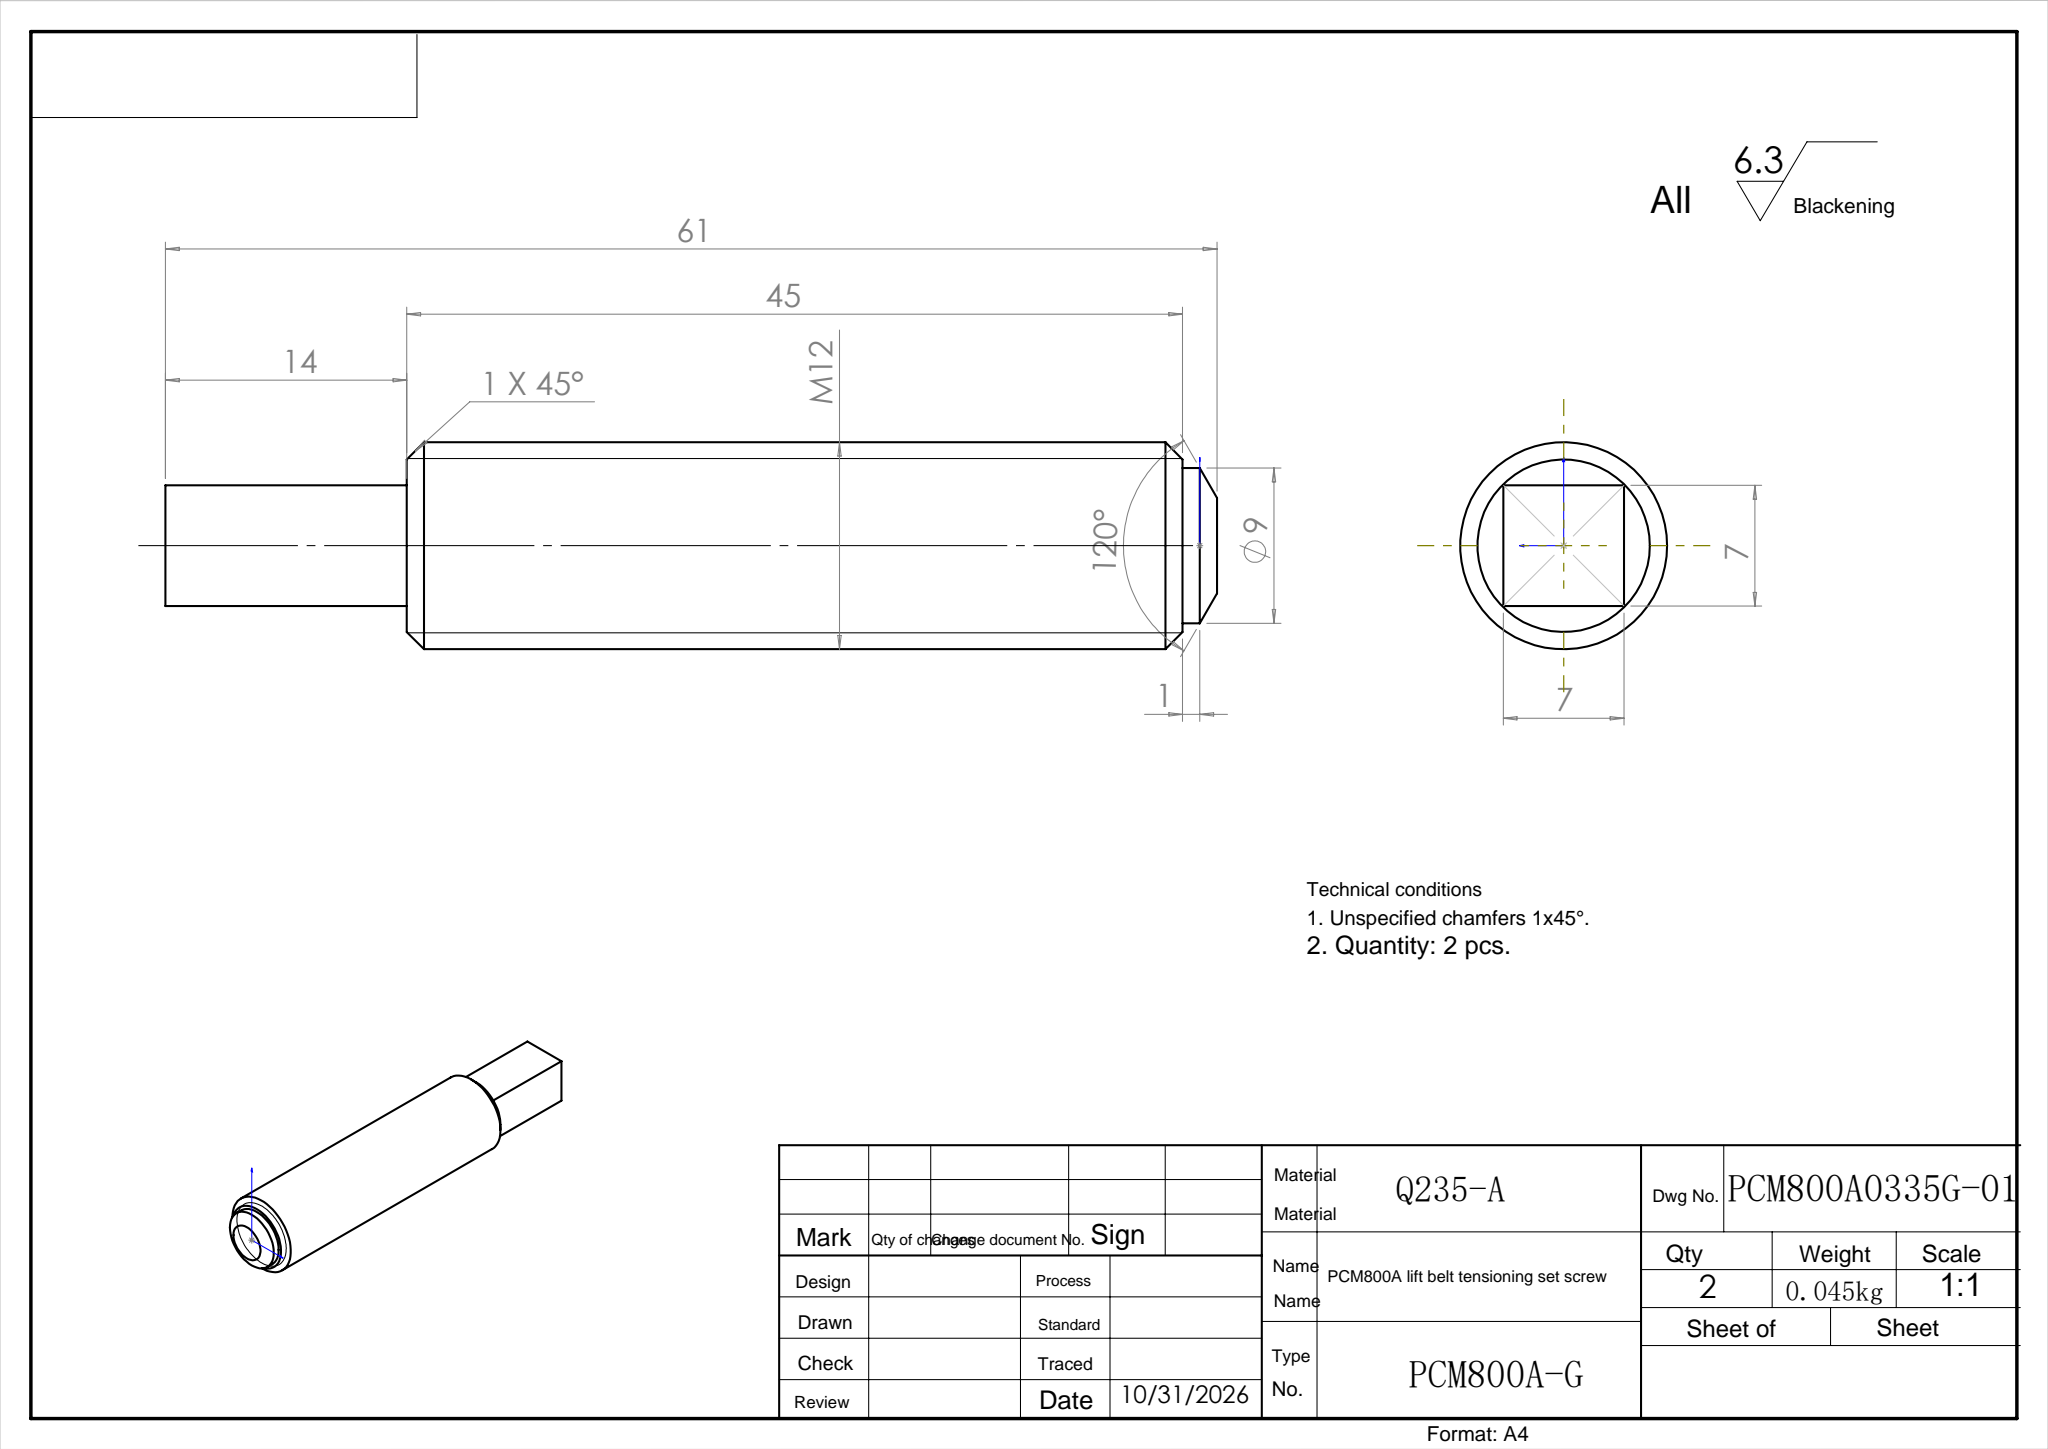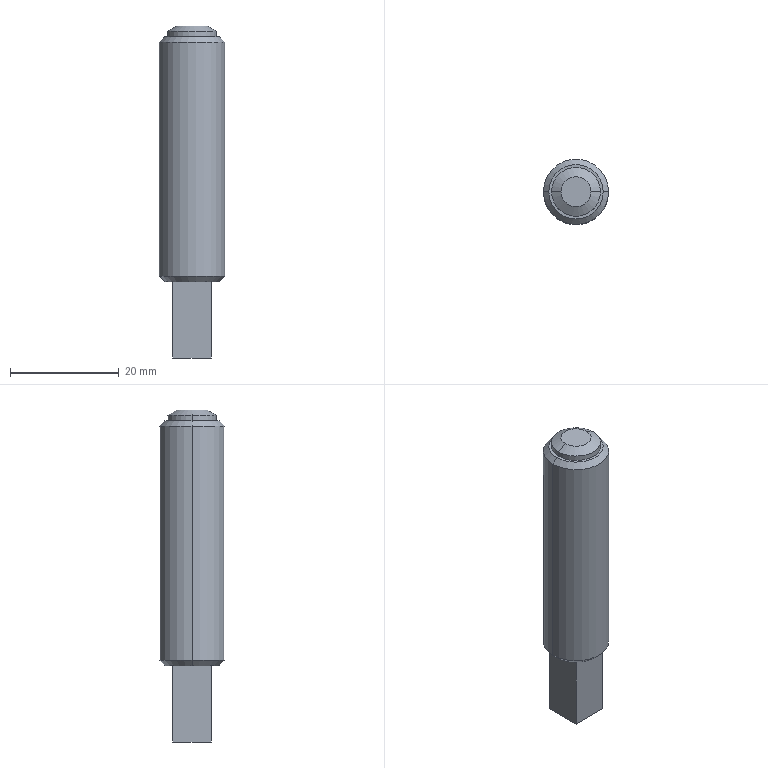Part | SolidWorks | features ICE 3, Chamfer 2, MirrorStock 1 | 1 solid | 18 faces | box 12 x 12 x 61 mm | volume 5846 mm3 | plane 8 | cone 6 | cylinder 4 | commonest cylinder face diameters 9 x2 12 x2
STEP:
#1=CARTESIAN_POINT('',(5.,0.,-1.));
#2=VERTEX_POINT('',#1);
#3=CARTESIAN_POINT('',(-5.,0.,-1.));
#4=VERTEX_POINT('',#3);
#5=CARTESIAN_POINT('',(0.,0.,-1.));
#6=DIRECTION('',(0.,0.,1.));
#7=DIRECTION('',(-1.,0.,0.));
#8=AXIS2_PLACEMENT_3D('',#5,#6,#7);
#9=CIRCLE('',#8,5.);
#10=EDGE_CURVE('',#2,#4,#9,.T.);
#11=ORIENTED_EDGE('',*,*,#10,.F.);
#12=CARTESIAN_POINT('',(6.,0.,-2.));
#13=VERTEX_POINT('',#12);
#14=CARTESIAN_POINT('',(5.,0.,-1.));
#15=DIRECTION('',(0.7071,0.,-0.7071));
#16=VECTOR('',#15,1000.);
#17=LINE('',#14,#16);
#18=EDGE_CURVE('',#2,#13,#17,.T.);
#19=ORIENTED_EDGE('',*,*,#18,.T.);
#20=CARTESIAN_POINT('',(-6.,0.,-2.));
#21=VERTEX_POINT('',#20);
#22=CARTESIAN_POINT('',(0.,0.,-2.));
#23=DIRECTION('',(0.,0.,-1.));
#24=DIRECTION('',(-1.,0.,0.));
#25=AXIS2_PLACEMENT_3D('',#22,#23,#24);
#26=CIRCLE('',#25,6.);
#27=EDGE_CURVE('',#21,#13,#26,.T.);
#28=ORIENTED_EDGE('',*,*,#27,.F.);
#29=CARTESIAN_POINT('',(-5.,0.,-1.));
#30=DIRECTION('',(-0.7071,0.,-0.7071));
#31=VECTOR('',#30,1000.);
#32=LINE('',#29,#31);
#33=EDGE_CURVE('',#4,#21,#32,.T.);
#34=ORIENTED_EDGE('',*,*,#33,.F.);
#35=EDGE_LOOP('',(#11,#19,#28,#34));
#36=FACE_OUTER_BOUND('',#35,.T.);
#37=CARTESIAN_POINT('',(0.,0.,-1.));
#38=DIRECTION('',(0.,0.,-1.));
#39=DIRECTION('',(-1.,0.,0.));
#40=AXIS2_PLACEMENT_3D('',#37,#38,#39);
#41=CONICAL_SURFACE('',#40,5.,0.7854);
#42=ADVANCED_FACE('',(#36),#41,.T.);
#43=CARTESIAN_POINT('',(-4.5,0.,-1.));
#44=VERTEX_POINT('',#43);
#45=CARTESIAN_POINT('',(4.5,0.,-1.));
#46=VERTEX_POINT('',#45);
#47=CARTESIAN_POINT('',(0.,0.,-1.));
#48=DIRECTION('',(0.,0.,1.));
#49=DIRECTION('',(1.,0.,0.));
#50=AXIS2_PLACEMENT_3D('',#47,#48,#49);
#51=CIRCLE('',#50,4.5);
#52=EDGE_CURVE('',#44,#46,#51,.T.);
#53=ORIENTED_EDGE('',*,*,#52,.T.);
#54=CARTESIAN_POINT('',(4.5,0.,0.));
#55=VERTEX_POINT('',#54);
#56=CARTESIAN_POINT('',(4.5,0.,-1.));
#57=DIRECTION('',(0.,0.,1.));
#58=VECTOR('',#57,1000.);
#59=LINE('',#56,#58);
#60=EDGE_CURVE('',#46,#55,#59,.T.);
#61=ORIENTED_EDGE('',*,*,#60,.T.);
#62=CARTESIAN_POINT('',(-4.5,0.,0.));
#63=VERTEX_POINT('',#62);
#64=CARTESIAN_POINT('',(0.,0.,0.));
#65=DIRECTION('',(0.,0.,-1.));
#66=DIRECTION('',(-1.,0.,0.));
#67=AXIS2_PLACEMENT_3D('',#64,#65,#66);
#68=CIRCLE('',#67,4.5);
#69=EDGE_CURVE('',#55,#63,#68,.T.);
#70=ORIENTED_EDGE('',*,*,#69,.T.);
#71=CARTESIAN_POINT('',(-4.5,0.,-1.));
#72=DIRECTION('',(0.,0.,1.));
#73=VECTOR('',#72,1000.);
#74=LINE('',#71,#73);
#75=EDGE_CURVE('',#44,#63,#74,.T.);
#76=ORIENTED_EDGE('',*,*,#75,.F.);
#77=EDGE_LOOP('',(#53,#61,#70,#76));
#78=FACE_OUTER_BOUND('',#77,.T.);
#79=CARTESIAN_POINT('',(0.,0.,-1.));
#80=DIRECTION('',(0.,0.,1.));
#81=DIRECTION('',(-1.,0.,0.));
#82=AXIS2_PLACEMENT_3D('',#79,#80,#81);
#83=CYLINDRICAL_SURFACE('',#82,4.5);
#84=ADVANCED_FACE('',(#78),#83,.T.);
#85=CARTESIAN_POINT('',(-2.768,0.,1.));
#86=VERTEX_POINT('',#85);
#87=CARTESIAN_POINT('',(2.768,0.,1.));
#88=VERTEX_POINT('',#87);
#89=CARTESIAN_POINT('',(0.,0.,1.));
#90=DIRECTION('',(0.,0.,-1.));
#91=DIRECTION('',(-1.,0.,0.));
#92=AXIS2_PLACEMENT_3D('',#89,#90,#91);
#93=CIRCLE('',#92,2.768);
#94=EDGE_CURVE('',#86,#88,#93,.T.);
#95=ORIENTED_EDGE('',*,*,#94,.T.);
#96=CARTESIAN_POINT('',(4.5,0.,0.));
#97=DIRECTION('',(0.866,0.,-0.5));
#98=VECTOR('',#97,1000.);
#99=LINE('',#96,#98);
#100=EDGE_CURVE('',#88,#55,#99,.T.);
#101=ORIENTED_EDGE('',*,*,#100,.T.);
#102=CARTESIAN_POINT('',(0.,0.,0.));
#103=DIRECTION('',(0.,0.,-1.));
#104=DIRECTION('',(-1.,0.,0.));
#105=AXIS2_PLACEMENT_3D('',#102,#103,#104);
#106=CIRCLE('',#105,4.5);
#107=EDGE_CURVE('',#63,#55,#106,.T.);
#108=ORIENTED_EDGE('',*,*,#107,.F.);
#109=CARTESIAN_POINT('',(-4.5,0.,0.));
#110=DIRECTION('',(-0.866,0.,-0.5));
#111=VECTOR('',#110,1000.);
#112=LINE('',#109,#111);
#113=EDGE_CURVE('',#86,#63,#112,.T.);
#114=ORIENTED_EDGE('',*,*,#113,.F.);
#115=EDGE_LOOP('',(#95,#101,#108,#114));
#116=FACE_OUTER_BOUND('',#115,.T.);
#117=CARTESIAN_POINT('',(0.,0.,0.));
#118=DIRECTION('',(0.,0.,-1.));
#119=DIRECTION('',(-1.,0.,0.));
#120=AXIS2_PLACEMENT_3D('',#117,#118,#119);
#121=CONICAL_SURFACE('',#120,4.5,1.047);
#122=ADVANCED_FACE('',(#116),#121,.T.);
#123=CARTESIAN_POINT('',(-5.,0.,-46.));
#124=VERTEX_POINT('',#123);
#125=CARTESIAN_POINT('',(5.,0.,-46.));
#126=VERTEX_POINT('',#125);
#127=CARTESIAN_POINT('',(0.,0.,-46.));
#128=DIRECTION('',(0.,0.,-1.));
#129=DIRECTION('',(-1.,0.,0.));
#130=AXIS2_PLACEMENT_3D('',#127,#128,#129);
#131=CIRCLE('',#130,5.);
#132=EDGE_CURVE('',#124,#126,#131,.T.);
#133=ORIENTED_EDGE('',*,*,#132,.F.);
#134=CARTESIAN_POINT('',(-6.,0.,-45.));
#135=VERTEX_POINT('',#134);
#136=CARTESIAN_POINT('',(-6.,0.,-45.));
#137=DIRECTION('',(-0.7071,0.,0.7071));
#138=VECTOR('',#137,1000.);
#139=LINE('',#136,#138);
#140=EDGE_CURVE('',#124,#135,#139,.T.);
#141=ORIENTED_EDGE('',*,*,#140,.T.);
#142=CARTESIAN_POINT('',(6.,0.,-45.));
#143=VERTEX_POINT('',#142);
#144=CARTESIAN_POINT('',(0.,0.,-45.));
#145=DIRECTION('',(0.,0.,1.));
#146=DIRECTION('',(-1.,0.,0.));
#147=AXIS2_PLACEMENT_3D('',#144,#145,#146);
#148=CIRCLE('',#147,6.);
#149=EDGE_CURVE('',#143,#135,#148,.T.);
#150=ORIENTED_EDGE('',*,*,#149,.F.);
#151=CARTESIAN_POINT('',(6.,0.,-45.));
#152=DIRECTION('',(0.7071,0.,0.7071));
#153=VECTOR('',#152,1000.);
#154=LINE('',#151,#153);
#155=EDGE_CURVE('',#126,#143,#154,.T.);
#156=ORIENTED_EDGE('',*,*,#155,.F.);
#157=EDGE_LOOP('',(#133,#141,#150,#156));
#158=FACE_OUTER_BOUND('',#157,.T.);
#159=CARTESIAN_POINT('',(0.,0.,-45.));
#160=DIRECTION('',(0.,0.,1.));
#161=DIRECTION('',(1.,0.,0.));
#162=AXIS2_PLACEMENT_3D('',#159,#160,#161);
#163=CONICAL_SURFACE('',#162,6.,0.7854);
#164=ADVANCED_FACE('',(#158),#163,.T.);
#165=CARTESIAN_POINT('',(0.,0.,-45.));
#166=DIRECTION('',(0.,0.,1.));
#167=DIRECTION('',(-1.,0.,0.));
#168=AXIS2_PLACEMENT_3D('',#165,#166,#167);
#169=CIRCLE('',#168,6.);
#170=EDGE_CURVE('',#135,#143,#169,.T.);
#171=ORIENTED_EDGE('',*,*,#170,.T.);
#172=CARTESIAN_POINT('',(6.,0.,-46.));
#173=DIRECTION('',(0.,0.,1.));
#174=VECTOR('',#173,1000.);
#175=LINE('',#172,#174);
#176=EDGE_CURVE('',#143,#13,#175,.T.);
#177=ORIENTED_EDGE('',*,*,#176,.T.);
#178=CARTESIAN_POINT('',(0.,0.,-2.));
#179=DIRECTION('',(0.,0.,-1.));
#180=DIRECTION('',(-1.,0.,0.));
#181=AXIS2_PLACEMENT_3D('',#178,#179,#180);
#182=CIRCLE('',#181,6.);
#183=EDGE_CURVE('',#13,#21,#182,.T.);
#184=ORIENTED_EDGE('',*,*,#183,.T.);
#185=CARTESIAN_POINT('',(-6.,0.,-46.));
#186=DIRECTION('',(0.,0.,1.));
#187=VECTOR('',#186,1000.);
#188=LINE('',#185,#187);
#189=EDGE_CURVE('',#135,#21,#188,.T.);
#190=ORIENTED_EDGE('',*,*,#189,.F.);
#191=EDGE_LOOP('',(#171,#177,#184,#190));
#192=FACE_OUTER_BOUND('',#191,.T.);
#193=CARTESIAN_POINT('',(0.,0.,-46.));
#194=DIRECTION('',(0.,0.,1.));
#195=DIRECTION('',(-1.,0.,0.));
#196=AXIS2_PLACEMENT_3D('',#193,#194,#195);
#197=CYLINDRICAL_SURFACE('',#196,6.);
#198=ADVANCED_FACE('',(#192),#197,.T.);
#199=CARTESIAN_POINT('',(0.,0.,-46.));
#200=DIRECTION('',(0.,0.,-1.));
#201=DIRECTION('',(-1.,0.,0.));
#202=AXIS2_PLACEMENT_3D('',#199,#200,#201);
#203=CIRCLE('',#202,5.);
#204=EDGE_CURVE('',#126,#124,#203,.T.);
#205=ORIENTED_EDGE('',*,*,#204,.T.);
#206=ORIENTED_EDGE('',*,*,#132,.T.);
#207=EDGE_LOOP('',(#205,#206));
#208=FACE_OUTER_BOUND('',#207,.T.);
#209=CARTESIAN_POINT('',(3.5,-3.5,-46.));
#210=VERTEX_POINT('',#209);
#211=CARTESIAN_POINT('',(-3.5,-3.5,-46.));
#212=VERTEX_POINT('',#211);
#213=CARTESIAN_POINT('',(3.5,-3.5,-46.));
#214=DIRECTION('',(-1.,0.,0.));
#215=VECTOR('',#214,1000.);
#216=LINE('',#213,#215);
#217=EDGE_CURVE('',#210,#212,#216,.T.);
#218=ORIENTED_EDGE('',*,*,#217,.F.);
#219=CARTESIAN_POINT('',(3.5,3.5,-46.));
#220=VERTEX_POINT('',#219);
#221=CARTESIAN_POINT('',(3.5,3.5,-46.));
#222=DIRECTION('',(0.,-1.,0.));
#223=VECTOR('',#222,1000.);
#224=LINE('',#221,#223);
#225=EDGE_CURVE('',#220,#210,#224,.T.);
#226=ORIENTED_EDGE('',*,*,#225,.F.);
#227=CARTESIAN_POINT('',(-3.5,3.5,-46.));
#228=VERTEX_POINT('',#227);
#229=CARTESIAN_POINT('',(3.5,3.5,-46.));
#230=DIRECTION('',(1.,0.,0.));
#231=VECTOR('',#230,1000.);
#232=LINE('',#229,#231);
#233=EDGE_CURVE('',#228,#220,#232,.T.);
#234=ORIENTED_EDGE('',*,*,#233,.F.);
#235=CARTESIAN_POINT('',(-3.5,3.5,-46.));
#236=DIRECTION('',(0.,1.,0.));
#237=VECTOR('',#236,1000.);
#238=LINE('',#235,#237);
#239=EDGE_CURVE('',#212,#228,#238,.T.);
#240=ORIENTED_EDGE('',*,*,#239,.F.);
#241=EDGE_LOOP('',(#218,#226,#234,#240));
#242=FACE_BOUND('',#241,.T.);
#243=CARTESIAN_POINT('',(0.,0.,-46.));
#244=DIRECTION('',(0.,0.,-1.));
#245=DIRECTION('',(1.,0.,0.));
#246=AXIS2_PLACEMENT_3D('',#243,#244,#245);
#247=PLANE('',#246);
#248=ADVANCED_FACE('',(#208,#242),#247,.T.);
#249=ORIENTED_EDGE('',*,*,#176,.F.);
#250=ORIENTED_EDGE('',*,*,#149,.T.);
#251=ORIENTED_EDGE('',*,*,#189,.T.);
#252=ORIENTED_EDGE('',*,*,#27,.T.);
#253=EDGE_LOOP('',(#249,#250,#251,#252));
#254=FACE_OUTER_BOUND('',#253,.T.);
#255=CARTESIAN_POINT('',(0.,0.,-46.));
#256=DIRECTION('',(0.,0.,1.));
#257=DIRECTION('',(-1.,0.,0.));
#258=AXIS2_PLACEMENT_3D('',#255,#256,#257);
#259=CYLINDRICAL_SURFACE('',#258,6.);
#260=ADVANCED_FACE('',(#254),#259,.T.);
#261=ORIENTED_EDGE('',*,*,#225,.T.);
#262=CARTESIAN_POINT('',(3.5,-3.5,-60.));
#263=VERTEX_POINT('',#262);
#264=CARTESIAN_POINT('',(3.5,-3.5,-60.));
#265=DIRECTION('',(0.,0.,1.));
#266=VECTOR('',#265,1000.);
#267=LINE('',#264,#266);
#268=EDGE_CURVE('',#263,#210,#267,.T.);
#269=ORIENTED_EDGE('',*,*,#268,.F.);
#270=CARTESIAN_POINT('',(3.5,3.5,-60.));
#271=VERTEX_POINT('',#270);
#272=CARTESIAN_POINT('',(3.5,3.5,-60.));
#273=DIRECTION('',(0.,-1.,0.));
#274=VECTOR('',#273,1000.);
#275=LINE('',#272,#274);
#276=EDGE_CURVE('',#271,#263,#275,.T.);
#277=ORIENTED_EDGE('',*,*,#276,.F.);
#278=CARTESIAN_POINT('',(3.5,3.5,-60.));
#279=DIRECTION('',(0.,0.,1.));
#280=VECTOR('',#279,1000.);
#281=LINE('',#278,#280);
#282=EDGE_CURVE('',#271,#220,#281,.T.);
#283=ORIENTED_EDGE('',*,*,#282,.T.);
#284=EDGE_LOOP('',(#261,#269,#277,#283));
#285=FACE_OUTER_BOUND('',#284,.T.);
#286=CARTESIAN_POINT('',(3.5,3.5,-60.));
#287=DIRECTION('',(-1.,0.,0.));
#288=DIRECTION('',(0.,-1.,0.));
#289=AXIS2_PLACEMENT_3D('',#286,#287,#288);
#290=PLANE('',#289);
#291=ADVANCED_FACE('',(#285),#290,.F.);
#292=ORIENTED_EDGE('',*,*,#217,.T.);
#293=CARTESIAN_POINT('',(-3.5,-3.5,-60.));
#294=VERTEX_POINT('',#293);
#295=CARTESIAN_POINT('',(-3.5,-3.5,-60.));
#296=DIRECTION('',(0.,0.,1.));
#297=VECTOR('',#296,1000.);
#298=LINE('',#295,#297);
#299=EDGE_CURVE('',#294,#212,#298,.T.);
#300=ORIENTED_EDGE('',*,*,#299,.F.);
#301=CARTESIAN_POINT('',(3.5,-3.5,-60.));
#302=DIRECTION('',(-1.,0.,0.));
#303=VECTOR('',#302,1000.);
#304=LINE('',#301,#303);
#305=EDGE_CURVE('',#263,#294,#304,.T.);
#306=ORIENTED_EDGE('',*,*,#305,.F.);
#307=ORIENTED_EDGE('',*,*,#268,.T.);
#308=EDGE_LOOP('',(#292,#300,#306,#307));
#309=FACE_OUTER_BOUND('',#308,.T.);
#310=CARTESIAN_POINT('',(3.5,-3.5,-60.));
#311=DIRECTION('',(0.,1.,0.));
#312=DIRECTION('',(0.,0.,1.));
#313=AXIS2_PLACEMENT_3D('',#310,#311,#312);
#314=PLANE('',#313);
#315=ADVANCED_FACE('',(#309),#314,.F.);
#316=ORIENTED_EDGE('',*,*,#239,.T.);
#317=CARTESIAN_POINT('',(-3.5,3.5,-60.));
#318=VERTEX_POINT('',#317);
#319=CARTESIAN_POINT('',(-3.5,3.5,-60.));
#320=DIRECTION('',(0.,0.,1.));
#321=VECTOR('',#320,1000.);
#322=LINE('',#319,#321);
#323=EDGE_CURVE('',#318,#228,#322,.T.);
#324=ORIENTED_EDGE('',*,*,#323,.F.);
#325=CARTESIAN_POINT('',(-3.5,3.5,-60.));
#326=DIRECTION('',(0.,1.,0.));
#327=VECTOR('',#326,1000.);
#328=LINE('',#325,#327);
#329=EDGE_CURVE('',#294,#318,#328,.T.);
#330=ORIENTED_EDGE('',*,*,#329,.F.);
#331=ORIENTED_EDGE('',*,*,#299,.T.);
#332=EDGE_LOOP('',(#316,#324,#330,#331));
#333=FACE_OUTER_BOUND('',#332,.T.);
#334=CARTESIAN_POINT('',(-3.5,3.5,-60.));
#335=DIRECTION('',(1.,0.,0.));
#336=DIRECTION('',(0.,1.,0.));
#337=AXIS2_PLACEMENT_3D('',#334,#335,#336);
#338=PLANE('',#337);
#339=ADVANCED_FACE('',(#333),#338,.F.);
#340=ORIENTED_EDGE('',*,*,#233,.T.);
#341=ORIENTED_EDGE('',*,*,#282,.F.);
#342=CARTESIAN_POINT('',(3.5,3.5,-60.));
#343=DIRECTION('',(1.,0.,0.));
#344=VECTOR('',#343,1000.);
#345=LINE('',#342,#344);
#346=EDGE_CURVE('',#318,#271,#345,.T.);
#347=ORIENTED_EDGE('',*,*,#346,.F.);
#348=ORIENTED_EDGE('',*,*,#323,.T.);
#349=EDGE_LOOP('',(#340,#341,#347,#348));
#350=FACE_OUTER_BOUND('',#349,.T.);
#351=CARTESIAN_POINT('',(3.5,3.5,-60.));
#352=DIRECTION('',(0.,-1.,0.));
#353=DIRECTION('',(0.,0.,-1.));
#354=AXIS2_PLACEMENT_3D('',#351,#352,#353);
#355=PLANE('',#354);
#356=ADVANCED_FACE('',(#350),#355,.F.);
#357=ORIENTED_EDGE('',*,*,#276,.T.);
#358=ORIENTED_EDGE('',*,*,#305,.T.);
#359=ORIENTED_EDGE('',*,*,#329,.T.);
#360=ORIENTED_EDGE('',*,*,#346,.T.);
#361=EDGE_LOOP('',(#357,#358,#359,#360));
#362=FACE_OUTER_BOUND('',#361,.T.);
#363=CARTESIAN_POINT('',(3.5,-3.5,-60.));
#364=DIRECTION('',(0.,0.,-1.));
#365=DIRECTION('',(-1.,0.,0.));
#366=AXIS2_PLACEMENT_3D('',#363,#364,#365);
#367=PLANE('',#366);
#368=ADVANCED_FACE('',(#362),#367,.T.);
#369=ORIENTED_EDGE('',*,*,#140,.F.);
#370=ORIENTED_EDGE('',*,*,#204,.F.);
#371=ORIENTED_EDGE('',*,*,#155,.T.);
#372=ORIENTED_EDGE('',*,*,#170,.F.);
#373=EDGE_LOOP('',(#369,#370,#371,#372));
#374=FACE_OUTER_BOUND('',#373,.T.);
#375=CARTESIAN_POINT('',(0.,0.,-45.));
#376=DIRECTION('',(0.,0.,1.));
#377=DIRECTION('',(1.,0.,0.));
#378=AXIS2_PLACEMENT_3D('',#375,#376,#377);
#379=CONICAL_SURFACE('',#378,6.,0.7854);
#380=ADVANCED_FACE('',(#374),#379,.T.);
#381=ORIENTED_EDGE('',*,*,#94,.F.);
#382=CARTESIAN_POINT('',(0.,0.,1.));
#383=DIRECTION('',(0.,0.,-1.));
#384=DIRECTION('',(-1.,0.,0.));
#385=AXIS2_PLACEMENT_3D('',#382,#383,#384);
#386=CIRCLE('',#385,2.768);
#387=EDGE_CURVE('',#88,#86,#386,.T.);
#388=ORIENTED_EDGE('',*,*,#387,.F.);
#389=EDGE_LOOP('',(#381,#388));
#390=FACE_OUTER_BOUND('',#389,.T.);
#391=CARTESIAN_POINT('',(0.,0.,1.));
#392=DIRECTION('',(0.,0.,1.));
#393=DIRECTION('',(-1.,0.,0.));
#394=AXIS2_PLACEMENT_3D('',#391,#392,#393);
#395=PLANE('',#394);
#396=ADVANCED_FACE('',(#390),#395,.T.);
#397=ORIENTED_EDGE('',*,*,#100,.F.);
#398=ORIENTED_EDGE('',*,*,#387,.T.);
#399=ORIENTED_EDGE('',*,*,#113,.T.);
#400=ORIENTED_EDGE('',*,*,#69,.F.);
#401=EDGE_LOOP('',(#397,#398,#399,#400));
#402=FACE_OUTER_BOUND('',#401,.T.);
#403=CARTESIAN_POINT('',(0.,0.,0.));
#404=DIRECTION('',(0.,0.,-1.));
#405=DIRECTION('',(-1.,0.,0.));
#406=AXIS2_PLACEMENT_3D('',#403,#404,#405);
#407=CONICAL_SURFACE('',#406,4.5,1.047);
#408=ADVANCED_FACE('',(#402),#407,.T.);
#409=ORIENTED_EDGE('',*,*,#60,.F.);
#410=CARTESIAN_POINT('',(0.,0.,-1.));
#411=DIRECTION('',(0.,0.,1.));
#412=DIRECTION('',(1.,0.,0.));
#413=AXIS2_PLACEMENT_3D('',#410,#411,#412);
#414=CIRCLE('',#413,4.5);
#415=EDGE_CURVE('',#46,#44,#414,.T.);
#416=ORIENTED_EDGE('',*,*,#415,.T.);
#417=ORIENTED_EDGE('',*,*,#75,.T.);
#418=ORIENTED_EDGE('',*,*,#107,.T.);
#419=EDGE_LOOP('',(#409,#416,#417,#418));
#420=FACE_OUTER_BOUND('',#419,.T.);
#421=CARTESIAN_POINT('',(0.,0.,-1.));
#422=DIRECTION('',(0.,0.,1.));
#423=DIRECTION('',(-1.,0.,0.));
#424=AXIS2_PLACEMENT_3D('',#421,#422,#423);
#425=CYLINDRICAL_SURFACE('',#424,4.5);
#426=ADVANCED_FACE('',(#420),#425,.T.);
#427=CARTESIAN_POINT('',(0.,0.,-1.));
#428=DIRECTION('',(0.,0.,1.));
#429=DIRECTION('',(-1.,0.,0.));
#430=AXIS2_PLACEMENT_3D('',#427,#428,#429);
#431=CIRCLE('',#430,5.);
#432=EDGE_CURVE('',#4,#2,#431,.T.);
#433=ORIENTED_EDGE('',*,*,#432,.T.);
#434=ORIENTED_EDGE('',*,*,#10,.T.);
#435=EDGE_LOOP('',(#433,#434));
#436=FACE_OUTER_BOUND('',#435,.T.);
#437=ORIENTED_EDGE('',*,*,#52,.F.);
#438=ORIENTED_EDGE('',*,*,#415,.F.);
#439=EDGE_LOOP('',(#437,#438));
#440=FACE_BOUND('',#439,.T.);
#441=CARTESIAN_POINT('',(0.,0.,-1.));
#442=DIRECTION('',(0.,0.,-1.));
#443=DIRECTION('',(1.,0.,0.));
#444=AXIS2_PLACEMENT_3D('',#441,#442,#443);
#445=PLANE('',#444);
#446=ADVANCED_FACE('',(#436,#440),#445,.F.);
#447=ORIENTED_EDGE('',*,*,#18,.F.);
#448=ORIENTED_EDGE('',*,*,#432,.F.);
#449=ORIENTED_EDGE('',*,*,#33,.T.);
#450=ORIENTED_EDGE('',*,*,#183,.F.);
#451=EDGE_LOOP('',(#447,#448,#449,#450));
#452=FACE_OUTER_BOUND('',#451,.T.);
#453=CARTESIAN_POINT('',(0.,0.,-1.));
#454=DIRECTION('',(0.,0.,-1.));
#455=DIRECTION('',(-1.,0.,0.));
#456=AXIS2_PLACEMENT_3D('',#453,#454,#455);
#457=CONICAL_SURFACE('',#456,5.,0.7854);
#458=ADVANCED_FACE('',(#452),#457,.T.);
#459=CLOSED_SHELL('',(#42,#84,#122,#164,#198,#248,#260,#291,#315,#339,#356,#368,#380,#396,#408,#426,#446,#458));
#460=MANIFOLD_SOLID_BREP('',#459);
#461=CARTESIAN_POINT('',(0.,0.,0.));
#462=DIRECTION('',(0.,0.,1.));
#463=DIRECTION('',(1.,0.,0.));
#464=AXIS2_PLACEMENT_3D('',#461,#462,#463);
#465=(LENGTH_UNIT()NAMED_UNIT(*)SI_UNIT(.MILLI.,.METRE.));
#466=UNCERTAINTY_MEASURE_WITH_UNIT(LENGTH_MEASURE(0.00001),#465,'','');
#467=(NAMED_UNIT(*)PLANE_ANGLE_UNIT()SI_UNIT($,.RADIAN.));
#468=(NAMED_UNIT(*)SI_UNIT($,.STERADIAN.)SOLID_ANGLE_UNIT());
#469=(GEOMETRIC_REPRESENTATION_CONTEXT(3)GLOBAL_UNCERTAINTY_ASSIGNED_CONTEXT((#466))GLOBAL_UNIT_ASSIGNED_CONTEXT((#465,#467,#468))REPRESENTATION_CONTEXT('',''));
#470=ADVANCED_BREP_SHAPE_REPRESENTATION('',(#460,#464),#469);